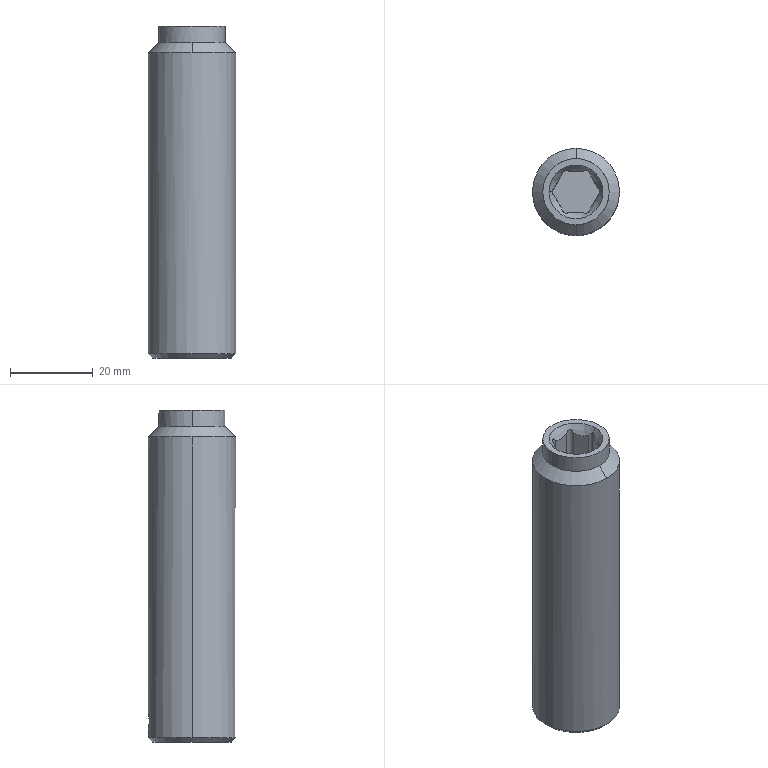Part | STEP file | Hex head-Mkt | 1 solid | 43 faces | box 21 x 21 x 80 mm | volume 24655 mm3 | cylinder 19 | plane 18 | cone 6 | commonest cylinder face diameters 2 x13 3.5 x2 16 x2 21 x2